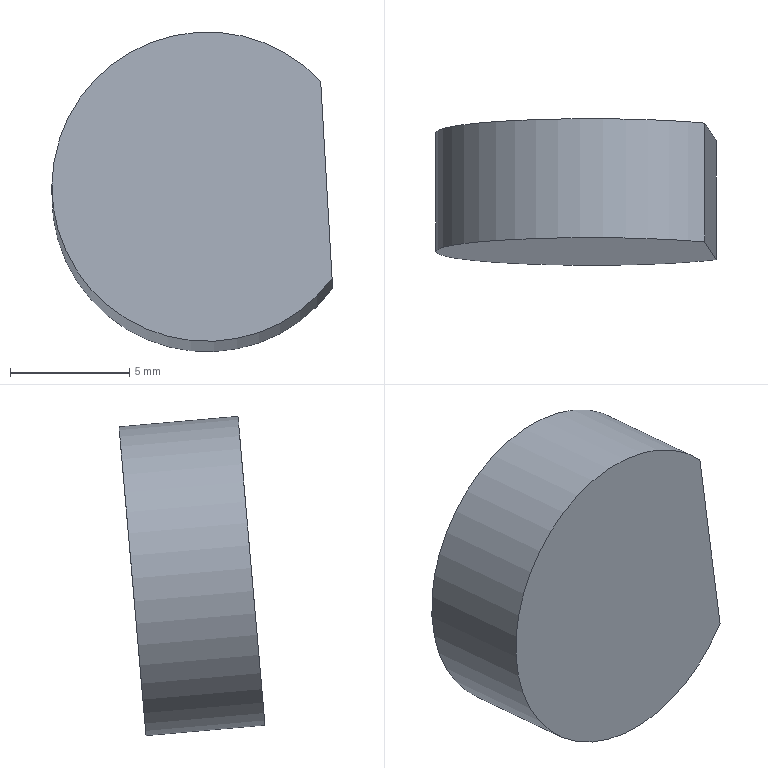Part | NX | features solid 2 | 1 solid | 4 faces | box 11.729 x 6.114 x 13.386 mm | volume 621.064 mm3 | plane 3 | cylinder 1 | commonest cylinder face diameters 13 x1
STEP:
#1=CARTESIAN_POINT('',(-223.612,-142.49,-20.126));
#2=VERTEX_POINT('',#1);
#3=CARTESIAN_POINT('',(-223.137,-143.213,-28.388));
#4=VERTEX_POINT('',#3);
#5=CARTESIAN_POINT('',(-223.375,-142.851,-24.257));
#6=DIRECTION('',(0.05719,-0.08701,-0.9946));
#7=VECTOR('',#6,1000.);
#8=LINE('',#5,#7);
#9=EDGE_CURVE('',#2,#4,#8,.T.);
#10=ORIENTED_EDGE('',*,*,#9,.F.);
#11=CARTESIAN_POINT('',(-228.366,-142.876,-24.542));
#12=DIRECTION('',(0.,-0.9962,0.08716));
#13=DIRECTION('',(0.,-0.08716,-0.9962));
#14=AXIS2_PLACEMENT_3D('',#11,#12,#13);
#15=CIRCLE('',#14,6.5);
#16=EDGE_CURVE('',#4,#2,#15,.F.);
#17=ORIENTED_EDGE('',*,*,#16,.F.);
#18=EDGE_LOOP('',(#10,#17));
#19=FACE_BOUND('',#18,.T.);
#20=CARTESIAN_POINT('',(-228.366,-142.876,-24.542));
#21=DIRECTION('',(0.,-0.9962,0.08716));
#22=DIRECTION('',(0.,-0.08716,-0.9962));
#23=AXIS2_PLACEMENT_3D('',#20,#21,#22);
#24=PLANE('',#23);
#25=ADVANCED_FACE('',(#19),#24,.T.);
#26=CARTESIAN_POINT('',(-223.137,-138.232,-28.823));
#27=VERTEX_POINT('',#26);
#28=CARTESIAN_POINT('',(-223.612,-137.509,-20.562));
#29=VERTEX_POINT('',#28);
#30=CARTESIAN_POINT('',(-223.375,-137.87,-24.693));
#31=DIRECTION('',(-0.05719,0.08701,0.9946));
#32=VECTOR('',#31,1000.);
#33=LINE('',#30,#32);
#34=EDGE_CURVE('',#27,#29,#33,.T.);
#35=ORIENTED_EDGE('',*,*,#34,.F.);
#36=CARTESIAN_POINT('',(-228.366,-137.895,-24.977));
#37=DIRECTION('',(0.,0.9962,-0.08716));
#38=DIRECTION('',(0.,0.08716,0.9962));
#39=AXIS2_PLACEMENT_3D('',#36,#37,#38);
#40=CIRCLE('',#39,6.5);
#41=EDGE_CURVE('',#29,#27,#40,.F.);
#42=ORIENTED_EDGE('',*,*,#41,.F.);
#43=EDGE_LOOP('',(#35,#42));
#44=FACE_BOUND('',#43,.T.);
#45=CARTESIAN_POINT('',(-228.366,-137.895,-24.977));
#46=DIRECTION('',(0.,0.9962,-0.08716));
#47=DIRECTION('',(0.,0.08716,0.9962));
#48=AXIS2_PLACEMENT_3D('',#45,#46,#47);
#49=PLANE('',#48);
#50=ADVANCED_FACE('',(#44),#49,.T.);
#51=CARTESIAN_POINT('',(-223.137,-128.27,-29.695));
#52=DIRECTION('',(0.,-0.9962,0.08716));
#53=VECTOR('',#52,1000.);
#54=LINE('',#51,#53);
#55=EDGE_CURVE('',#4,#27,#54,.F.);
#56=ORIENTED_EDGE('',*,*,#55,.F.);
#57=ORIENTED_EDGE('',*,*,#16,.T.);
#58=CARTESIAN_POINT('',(-223.612,-127.547,-21.433));
#59=DIRECTION('',(0.,-0.9962,0.08716));
#60=VECTOR('',#59,1000.);
#61=LINE('',#58,#60);
#62=EDGE_CURVE('',#29,#2,#61,.T.);
#63=ORIENTED_EDGE('',*,*,#62,.F.);
#64=ORIENTED_EDGE('',*,*,#41,.T.);
#65=EDGE_LOOP('',(#56,#57,#63,#64));
#66=FACE_BOUND('',#65,.T.);
#67=CARTESIAN_POINT('',(-228.366,-127.933,-25.849));
#68=DIRECTION('',(0.,-0.9962,0.08716));
#69=DIRECTION('',(0.,-0.08716,-0.9962));
#70=AXIS2_PLACEMENT_3D('',#67,#68,#69);
#71=CYLINDRICAL_SURFACE('',#70,6.5);
#72=ADVANCED_FACE('',(#66),#71,.T.);
#73=ORIENTED_EDGE('',*,*,#55,.T.);
#74=ORIENTED_EDGE('',*,*,#34,.T.);
#75=ORIENTED_EDGE('',*,*,#62,.T.);
#76=ORIENTED_EDGE('',*,*,#9,.T.);
#77=EDGE_LOOP('',(#73,#74,#75,#76));
#78=FACE_BOUND('',#77,.T.);
#79=CARTESIAN_POINT('',(-223.317,-126.999,-26.646));
#80=DIRECTION('',(-0.9984,-0.004985,-0.05697));
#81=DIRECTION('',(0.,-0.9962,0.08716));
#82=AXIS2_PLACEMENT_3D('',#79,#80,#81);
#83=PLANE('',#82);
#84=ADVANCED_FACE('',(#78),#83,.F.);
#85=CLOSED_SHELL('',(#25,#50,#72,#84));
#86=MANIFOLD_SOLID_BREP('',#85);
#87=(LENGTH_UNIT()NAMED_UNIT(*)SI_UNIT(.MILLI.,.METRE.));
#88=UNCERTAINTY_MEASURE_WITH_UNIT(LENGTH_MEASURE(0.00001),#87,'','');
#89=(NAMED_UNIT(*)PLANE_ANGLE_UNIT()SI_UNIT($,.RADIAN.));
#90=(NAMED_UNIT(*)SI_UNIT($,.STERADIAN.)SOLID_ANGLE_UNIT());
#91=(GEOMETRIC_REPRESENTATION_CONTEXT(3)GLOBAL_UNCERTAINTY_ASSIGNED_CONTEXT((#88))GLOBAL_UNIT_ASSIGNED_CONTEXT((#87,#89,#90))REPRESENTATION_CONTEXT('',''));
#92=ADVANCED_BREP_SHAPE_REPRESENTATION('',(#86),#91);